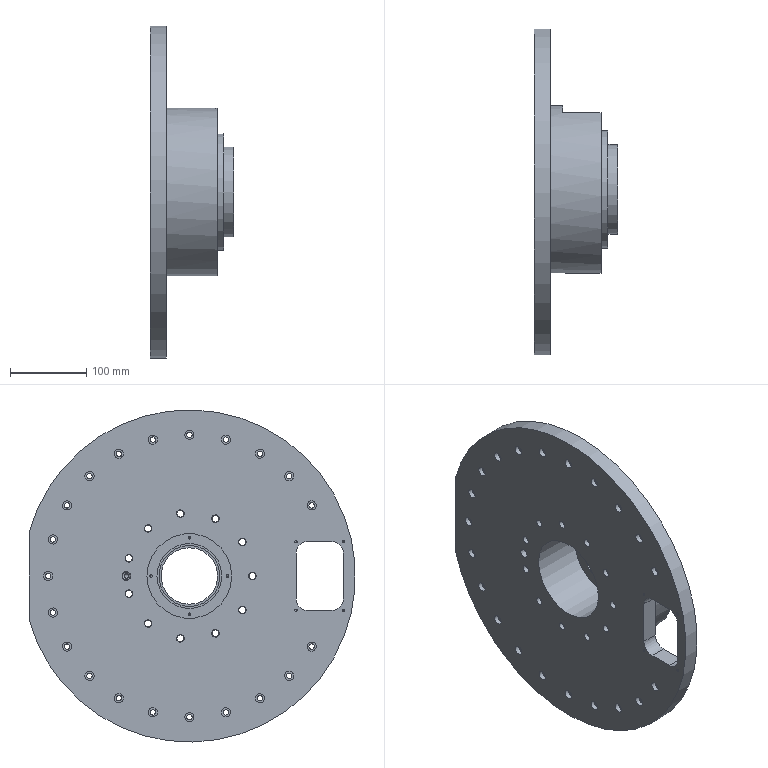Part | STEP file | Lower housing part | 1 solid | 171 faces | box 109.5 x 427.5 x 435 mm | volume 4806369 mm3 | cylinder 99 | plane 40 | cone 32 | commonest cylinder face diameters 7 x21 12 x21 9 x11 10 x11 3.242 x8 4.917 x8